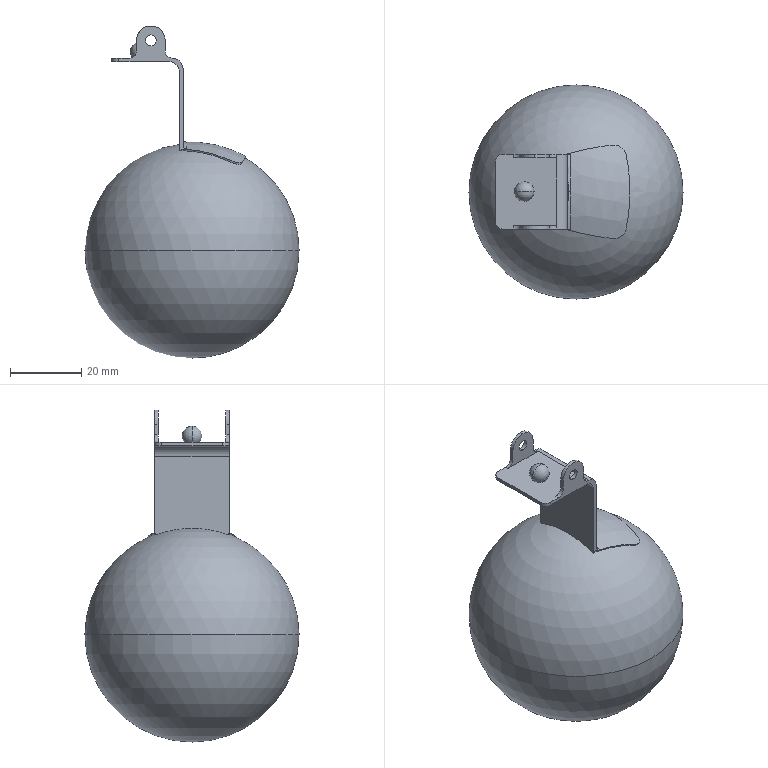Part | SolidWorks | features Fillet 5, ICE 3, Revolution 3, MirrorPattern 1 | 1 solid | 61 faces | box 60 x 60 x 93.006 mm | volume 12285 mm3 | plane 24 | cylinder 15 | sphere 10 | cone 6 | torus 4 | spline 2 | commonest cylinder face diameters 4 x6 3 x4 8 x3 6 x2